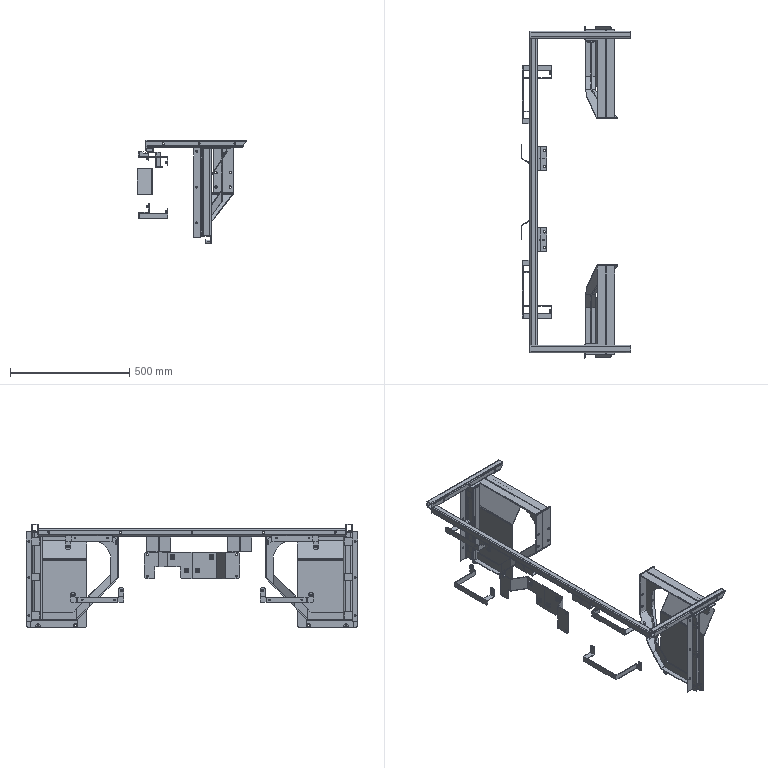Part | NX | features BREP 60 | 44 solids | 1333 faces | box 460.374 x 1390 x 435 mm | volume 2769143 mm3 | plane 819 | cylinder 412 | cone 96 | spline 6 | commonest cylinder face diameters 8 x168 10 x54 6 x40 16 x32 7 x24 7.5 x16